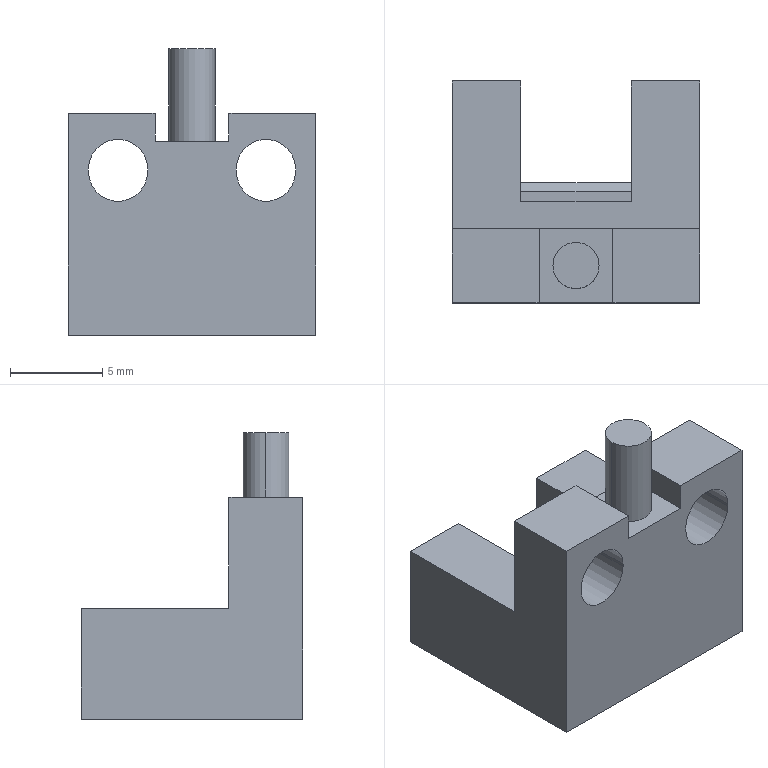Part | SolidWorks | features ICE 1, MBimport 1, MoveFace 1 | 1 solid | 43 faces | box 13.4 x 12 x 15.5 mm | volume 1013 mm3 | plane 37 | cylinder 6 | commonest cylinder face diameters 3.2 x4 2.5 x2
STEP:
#1=CARTESIAN_POINT('',(1.75,-8.,12.5));
#2=VERTEX_POINT('',#1);
#3=CARTESIAN_POINT('',(1.75,-8.,7.5));
#4=VERTEX_POINT('',#3);
#5=CARTESIAN_POINT('',(1.75,-8.,57.5));
#6=DIRECTION('',(0.,0.,-1.));
#7=VECTOR('',#6,1000.);
#8=LINE('',#5,#7);
#9=EDGE_CURVE('',#2,#4,#8,.T.);
#10=ORIENTED_EDGE('',*,*,#9,.F.);
#11=CARTESIAN_POINT('',(4.25,-8.,12.5));
#12=VERTEX_POINT('',#11);
#13=CARTESIAN_POINT('',(3.,-8.,12.5));
#14=DIRECTION('',(0.,0.,1.));
#15=DIRECTION('',(1.,0.,0.));
#16=AXIS2_PLACEMENT_3D('',#13,#14,#15);
#17=CIRCLE('',#16,1.25);
#18=EDGE_CURVE('',#12,#2,#17,.T.);
#19=ORIENTED_EDGE('',*,*,#18,.F.);
#20=CARTESIAN_POINT('',(4.25,-8.,7.5));
#21=VERTEX_POINT('',#20);
#22=CARTESIAN_POINT('',(4.25,-8.,57.5));
#23=DIRECTION('',(0.,0.,-1.));
#24=VECTOR('',#23,1000.);
#25=LINE('',#22,#24);
#26=EDGE_CURVE('',#12,#21,#25,.T.);
#27=ORIENTED_EDGE('',*,*,#26,.T.);
#28=CARTESIAN_POINT('',(3.,-8.,7.5));
#29=DIRECTION('',(0.,0.,1.));
#30=DIRECTION('',(-1.,0.,0.));
#31=AXIS2_PLACEMENT_3D('',#28,#29,#30);
#32=CIRCLE('',#31,1.25);
#33=EDGE_CURVE('',#21,#4,#32,.T.);
#34=ORIENTED_EDGE('',*,*,#33,.T.);
#35=EDGE_LOOP('',(#10,#19,#27,#34));
#36=FACE_OUTER_BOUND('',#35,.T.);
#37=CARTESIAN_POINT('',(3.,-8.,57.5));
#38=DIRECTION('',(0.,0.,-1.));
#39=DIRECTION('',(-1.,0.,0.));
#40=AXIS2_PLACEMENT_3D('',#37,#38,#39);
#41=CYLINDRICAL_SURFACE('',#40,1.25);
#42=ADVANCED_FACE('',(#36),#41,.T.);
#43=ORIENTED_EDGE('',*,*,#26,.F.);
#44=CARTESIAN_POINT('',(3.,-8.,12.5));
#45=DIRECTION('',(0.,0.,1.));
#46=DIRECTION('',(1.,0.,0.));
#47=AXIS2_PLACEMENT_3D('',#44,#45,#46);
#48=CIRCLE('',#47,1.25);
#49=EDGE_CURVE('',#2,#12,#48,.T.);
#50=ORIENTED_EDGE('',*,*,#49,.F.);
#51=ORIENTED_EDGE('',*,*,#9,.T.);
#52=CARTESIAN_POINT('',(3.,-8.,7.5));
#53=DIRECTION('',(0.,0.,1.));
#54=DIRECTION('',(-1.,0.,0.));
#55=AXIS2_PLACEMENT_3D('',#52,#53,#54);
#56=CIRCLE('',#55,1.25);
#57=EDGE_CURVE('',#4,#21,#56,.T.);
#58=ORIENTED_EDGE('',*,*,#57,.T.);
#59=EDGE_LOOP('',(#43,#50,#51,#58));
#60=FACE_OUTER_BOUND('',#59,.T.);
#61=CARTESIAN_POINT('',(3.,-8.,57.5));
#62=DIRECTION('',(0.,0.,-1.));
#63=DIRECTION('',(-1.,0.,0.));
#64=AXIS2_PLACEMENT_3D('',#61,#62,#63);
#65=CYLINDRICAL_SURFACE('',#64,1.25);
#66=ADVANCED_FACE('',(#60),#65,.T.);
#67=CARTESIAN_POINT('',(5.,-6.,7.5));
#68=VERTEX_POINT('',#67);
#69=CARTESIAN_POINT('',(1.,-6.,7.5));
#70=VERTEX_POINT('',#69);
#71=CARTESIAN_POINT('',(1.,-6.,7.5));
#72=DIRECTION('',(-1.,0.,0.));
#73=VECTOR('',#72,1000.);
#74=LINE('',#71,#73);
#75=EDGE_CURVE('',#68,#70,#74,.T.);
#76=ORIENTED_EDGE('',*,*,#75,.T.);
#77=CARTESIAN_POINT('',(1.,-10.,7.5));
#78=VERTEX_POINT('',#77);
#79=CARTESIAN_POINT('',(1.,-10.,7.5));
#80=DIRECTION('',(0.,1.,0.));
#81=VECTOR('',#80,1000.);
#82=LINE('',#79,#81);
#83=EDGE_CURVE('',#78,#70,#82,.T.);
#84=ORIENTED_EDGE('',*,*,#83,.F.);
#85=CARTESIAN_POINT('',(5.,-10.,7.5));
#86=VERTEX_POINT('',#85);
#87=CARTESIAN_POINT('',(1.,-10.,7.5));
#88=DIRECTION('',(-1.,0.,0.));
#89=VECTOR('',#88,1000.);
#90=LINE('',#87,#89);
#91=EDGE_CURVE('',#86,#78,#90,.T.);
#92=ORIENTED_EDGE('',*,*,#91,.F.);
#93=CARTESIAN_POINT('',(5.,-10.,7.5));
#94=DIRECTION('',(0.,1.,0.));
#95=VECTOR('',#94,1000.);
#96=LINE('',#93,#95);
#97=EDGE_CURVE('',#86,#68,#96,.T.);
#98=ORIENTED_EDGE('',*,*,#97,.T.);
#99=EDGE_LOOP('',(#76,#84,#92,#98));
#100=FACE_OUTER_BOUND('',#99,.T.);
#101=ORIENTED_EDGE('',*,*,#57,.F.);
#102=ORIENTED_EDGE('',*,*,#33,.F.);
#103=EDGE_LOOP('',(#101,#102));
#104=FACE_BOUND('',#103,.T.);
#105=CARTESIAN_POINT('',(1.,-10.,7.5));
#106=DIRECTION('',(0.,0.,-1.));
#107=DIRECTION('',(0.,-1.,0.));
#108=AXIS2_PLACEMENT_3D('',#105,#106,#107);
#109=PLANE('',#108);
#110=ADVANCED_FACE('',(#100,#104),#109,.F.);
#111=CARTESIAN_POINT('',(5.,-10.,9.));
#112=VERTEX_POINT('',#111);
#113=CARTESIAN_POINT('',(5.,-6.,9.));
#114=VERTEX_POINT('',#113);
#115=CARTESIAN_POINT('',(5.,-10.,9.));
#116=DIRECTION('',(0.,1.,0.));
#117=VECTOR('',#116,1000.);
#118=LINE('',#115,#117);
#119=EDGE_CURVE('',#112,#114,#118,.T.);
#120=ORIENTED_EDGE('',*,*,#119,.F.);
#121=CARTESIAN_POINT('',(9.7,-10.,9.));
#122=VERTEX_POINT('',#121);
#123=CARTESIAN_POINT('',(9.7,-10.,9.));
#124=DIRECTION('',(1.,0.,0.));
#125=VECTOR('',#124,1000.);
#126=LINE('',#123,#125);
#127=EDGE_CURVE('',#112,#122,#126,.T.);
#128=ORIENTED_EDGE('',*,*,#127,.T.);
#129=CARTESIAN_POINT('',(9.7,-6.,9.));
#130=VERTEX_POINT('',#129);
#131=CARTESIAN_POINT('',(9.7,-10.,9.));
#132=DIRECTION('',(0.,1.,0.));
#133=VECTOR('',#132,1000.);
#134=LINE('',#131,#133);
#135=EDGE_CURVE('',#122,#130,#134,.T.);
#136=ORIENTED_EDGE('',*,*,#135,.T.);
#137=CARTESIAN_POINT('',(9.7,-6.,9.));
#138=DIRECTION('',(-1.,0.,0.));
#139=VECTOR('',#138,1000.);
#140=LINE('',#137,#139);
#141=EDGE_CURVE('',#130,#114,#140,.T.);
#142=ORIENTED_EDGE('',*,*,#141,.T.);
#143=EDGE_LOOP('',(#120,#128,#136,#142));
#144=FACE_OUTER_BOUND('',#143,.T.);
#145=CARTESIAN_POINT('',(9.7,-6.,9.));
#146=DIRECTION('',(0.,0.,1.));
#147=DIRECTION('',(1.,0.,0.));
#148=AXIS2_PLACEMENT_3D('',#145,#146,#147);
#149=PLANE('',#148);
#150=ADVANCED_FACE('',(#144),#149,.T.);
#151=CARTESIAN_POINT('',(0.,-4.5,-3.));
#152=VERTEX_POINT('',#151);
#153=CARTESIAN_POINT('',(0.,2.,-3.));
#154=VERTEX_POINT('',#153);
#155=CARTESIAN_POINT('',(0.,-3.5,-3.));
#156=DIRECTION('',(0.,1.,0.));
#157=VECTOR('',#156,1000.);
#158=LINE('',#155,#157);
#159=EDGE_CURVE('',#152,#154,#158,.T.);
#160=ORIENTED_EDGE('',*,*,#159,.T.);
#161=CARTESIAN_POINT('',(0.,2.,3.));
#162=VERTEX_POINT('',#161);
#163=CARTESIAN_POINT('',(0.,2.,3.));
#164=DIRECTION('',(0.,0.,-1.));
#165=VECTOR('',#164,1000.);
#166=LINE('',#163,#165);
#167=EDGE_CURVE('',#162,#154,#166,.T.);
#168=ORIENTED_EDGE('',*,*,#167,.F.);
#169=CARTESIAN_POINT('',(0.,-4.5,3.));
#170=VERTEX_POINT('',#169);
#171=CARTESIAN_POINT('',(0.,-3.5,3.));
#172=DIRECTION('',(0.,1.,0.));
#173=VECTOR('',#172,1000.);
#174=LINE('',#171,#173);
#175=EDGE_CURVE('',#170,#162,#174,.T.);
#176=ORIENTED_EDGE('',*,*,#175,.F.);
#177=CARTESIAN_POINT('',(0.,-4.5,2.5));
#178=VERTEX_POINT('',#177);
#179=CARTESIAN_POINT('',(0.,-4.5,3.));
#180=DIRECTION('',(0.,0.,1.));
#181=VECTOR('',#180,1000.);
#182=LINE('',#179,#181);
#183=EDGE_CURVE('',#178,#170,#182,.T.);
#184=ORIENTED_EDGE('',*,*,#183,.F.);
#185=CARTESIAN_POINT('',(0.,-4.,2.5));
#186=VERTEX_POINT('',#185);
#187=CARTESIAN_POINT('',(0.,-4.5,2.5));
#188=DIRECTION('',(0.,1.,0.));
#189=VECTOR('',#188,1000.);
#190=LINE('',#187,#189);
#191=EDGE_CURVE('',#178,#186,#190,.T.);
#192=ORIENTED_EDGE('',*,*,#191,.T.);
#193=CARTESIAN_POINT('',(0.,-3.5,2.));
#194=VERTEX_POINT('',#193);
#195=CARTESIAN_POINT('',(0.,-4.,2.5));
#196=DIRECTION('',(0.,0.7071,-0.7071));
#197=VECTOR('',#196,1000.);
#198=LINE('',#195,#197);
#199=EDGE_CURVE('',#186,#194,#198,.T.);
#200=ORIENTED_EDGE('',*,*,#199,.T.);
#201=CARTESIAN_POINT('',(0.,-3.5,-2.));
#202=VERTEX_POINT('',#201);
#203=CARTESIAN_POINT('',(0.,-3.5,3.));
#204=DIRECTION('',(0.,0.,-1.));
#205=VECTOR('',#204,1000.);
#206=LINE('',#203,#205);
#207=EDGE_CURVE('',#194,#202,#206,.T.);
#208=ORIENTED_EDGE('',*,*,#207,.T.);
#209=CARTESIAN_POINT('',(0.,-4.,-2.5));
#210=VERTEX_POINT('',#209);
#211=CARTESIAN_POINT('',(0.,-1.,0.5));
#212=DIRECTION('',(0.,-0.7071,-0.7071));
#213=VECTOR('',#212,1000.);
#214=LINE('',#211,#213);
#215=EDGE_CURVE('',#202,#210,#214,.T.);
#216=ORIENTED_EDGE('',*,*,#215,.T.);
#217=CARTESIAN_POINT('',(0.,-4.5,-2.5));
#218=VERTEX_POINT('',#217);
#219=CARTESIAN_POINT('',(0.,-4.5,-2.5));
#220=DIRECTION('',(0.,1.,0.));
#221=VECTOR('',#220,1000.);
#222=LINE('',#219,#221);
#223=EDGE_CURVE('',#218,#210,#222,.T.);
#224=ORIENTED_EDGE('',*,*,#223,.F.);
#225=CARTESIAN_POINT('',(0.,-4.5,-3.));
#226=DIRECTION('',(0.,0.,1.));
#227=VECTOR('',#226,1000.);
#228=LINE('',#225,#227);
#229=EDGE_CURVE('',#152,#218,#228,.T.);
#230=ORIENTED_EDGE('',*,*,#229,.F.);
#231=EDGE_LOOP('',(#160,#168,#176,#184,#192,#200,#208,#216,#224,#230));
#232=FACE_OUTER_BOUND('',#231,.T.);
#233=CARTESIAN_POINT('',(0.,-0.6,0.4));
#234=VERTEX_POINT('',#233);
#235=CARTESIAN_POINT('',(0.,-0.6,-0.4));
#236=VERTEX_POINT('',#235);
#237=CARTESIAN_POINT('',(0.,-0.6,0.4));
#238=DIRECTION('',(0.,0.,-1.));
#239=VECTOR('',#238,1000.);
#240=LINE('',#237,#239);
#241=EDGE_CURVE('',#234,#236,#240,.T.);
#242=ORIENTED_EDGE('',*,*,#241,.F.);
#243=CARTESIAN_POINT('',(0.,0.6,0.4));
#244=VERTEX_POINT('',#243);
#245=CARTESIAN_POINT('',(0.,-0.6,0.4));
#246=DIRECTION('',(0.,-1.,0.));
#247=VECTOR('',#246,1000.);
#248=LINE('',#245,#247);
#249=EDGE_CURVE('',#244,#234,#248,.T.);
#250=ORIENTED_EDGE('',*,*,#249,.F.);
#251=CARTESIAN_POINT('',(0.,0.6,-0.4));
#252=VERTEX_POINT('',#251);
#253=CARTESIAN_POINT('',(0.,0.6,0.4));
#254=DIRECTION('',(0.,0.,1.));
#255=VECTOR('',#254,1000.);
#256=LINE('',#253,#255);
#257=EDGE_CURVE('',#252,#244,#256,.T.);
#258=ORIENTED_EDGE('',*,*,#257,.F.);
#259=CARTESIAN_POINT('',(0.,-0.6,-0.4));
#260=DIRECTION('',(0.,1.,0.));
#261=VECTOR('',#260,1000.);
#262=LINE('',#259,#261);
#263=EDGE_CURVE('',#236,#252,#262,.T.);
#264=ORIENTED_EDGE('',*,*,#263,.F.);
#265=EDGE_LOOP('',(#242,#250,#258,#264));
#266=FACE_BOUND('',#265,.T.);
#267=CARTESIAN_POINT('',(0.,-3.5,3.));
#268=DIRECTION('',(-1.,0.,0.));
#269=DIRECTION('',(0.,0.,1.));
#270=AXIS2_PLACEMENT_3D('',#267,#268,#269);
#271=PLANE('',#270);
#272=ADVANCED_FACE('',(#232,#266),#271,.F.);
#273=CARTESIAN_POINT('',(-3.7,2.,-3.));
#274=VERTEX_POINT('',#273);
#275=CARTESIAN_POINT('',(0.,2.,-3.));
#276=DIRECTION('',(-1.,0.,0.));
#277=VECTOR('',#276,1000.);
#278=LINE('',#275,#277);
#279=EDGE_CURVE('',#154,#274,#278,.T.);
#280=ORIENTED_EDGE('',*,*,#279,.T.);
#281=CARTESIAN_POINT('',(-3.7,2.,3.));
#282=VERTEX_POINT('',#281);
#283=CARTESIAN_POINT('',(-3.7,2.,3.));
#284=DIRECTION('',(0.,0.,-1.));
#285=VECTOR('',#284,1000.);
#286=LINE('',#283,#285);
#287=EDGE_CURVE('',#282,#274,#286,.T.);
#288=ORIENTED_EDGE('',*,*,#287,.F.);
#289=CARTESIAN_POINT('',(0.,2.,3.));
#290=DIRECTION('',(-1.,0.,0.));
#291=VECTOR('',#290,1000.);
#292=LINE('',#289,#291);
#293=EDGE_CURVE('',#162,#282,#292,.T.);
#294=ORIENTED_EDGE('',*,*,#293,.F.);
#295=ORIENTED_EDGE('',*,*,#167,.T.);
#296=EDGE_LOOP('',(#280,#288,#294,#295));
#297=FACE_OUTER_BOUND('',#296,.T.);
#298=CARTESIAN_POINT('',(0.,2.,3.));
#299=DIRECTION('',(0.,-1.,0.));
#300=DIRECTION('',(0.,0.,-1.));
#301=AXIS2_PLACEMENT_3D('',#298,#299,#300);
#302=PLANE('',#301);
#303=ADVANCED_FACE('',(#297),#302,.F.);
#304=CARTESIAN_POINT('',(-3.7,-10.,-3.));
#305=VERTEX_POINT('',#304);
#306=CARTESIAN_POINT('',(-3.7,2.,-3.));
#307=DIRECTION('',(0.,-1.,0.));
#308=VECTOR('',#307,1000.);
#309=LINE('',#306,#308);
#310=EDGE_CURVE('',#274,#305,#309,.T.);
#311=ORIENTED_EDGE('',*,*,#310,.T.);
#312=CARTESIAN_POINT('',(-3.7,-10.,9.));
#313=VERTEX_POINT('',#312);
#314=CARTESIAN_POINT('',(-3.7,-10.,3.));
#315=DIRECTION('',(0.,0.,-1.));
#316=VECTOR('',#315,1000.);
#317=LINE('',#314,#316);
#318=EDGE_CURVE('',#313,#305,#317,.T.);
#319=ORIENTED_EDGE('',*,*,#318,.F.);
#320=CARTESIAN_POINT('',(-3.7,-6.,9.));
#321=VERTEX_POINT('',#320);
#322=CARTESIAN_POINT('',(-3.7,-10.,9.));
#323=DIRECTION('',(0.,-1.,0.));
#324=VECTOR('',#323,1000.);
#325=LINE('',#322,#324);
#326=EDGE_CURVE('',#321,#313,#325,.T.);
#327=ORIENTED_EDGE('',*,*,#326,.F.);
#328=CARTESIAN_POINT('',(-3.7,-6.,3.));
#329=VERTEX_POINT('',#328);
#330=CARTESIAN_POINT('',(-3.7,-6.,9.));
#331=DIRECTION('',(0.,0.,-1.));
#332=VECTOR('',#331,1000.);
#333=LINE('',#330,#332);
#334=EDGE_CURVE('',#321,#329,#333,.T.);
#335=ORIENTED_EDGE('',*,*,#334,.T.);
#336=CARTESIAN_POINT('',(-3.7,2.,3.));
#337=DIRECTION('',(0.,-1.,0.));
#338=VECTOR('',#337,1000.);
#339=LINE('',#336,#338);
#340=EDGE_CURVE('',#282,#329,#339,.T.);
#341=ORIENTED_EDGE('',*,*,#340,.F.);
#342=ORIENTED_EDGE('',*,*,#287,.T.);
#343=EDGE_LOOP('',(#311,#319,#327,#335,#341,#342));
#344=FACE_OUTER_BOUND('',#343,.T.);
#345=CARTESIAN_POINT('',(-3.7,2.,3.));
#346=DIRECTION('',(1.,0.,0.));
#347=DIRECTION('',(0.,1.,0.));
#348=AXIS2_PLACEMENT_3D('',#345,#346,#347);
#349=PLANE('',#348);
#350=ADVANCED_FACE('',(#344),#349,.F.);
#351=ORIENTED_EDGE('',*,*,#127,.F.);
#352=CARTESIAN_POINT('',(5.,-10.,9.));
#353=DIRECTION('',(0.,0.,-1.));
#354=VECTOR('',#353,1000.);
#355=LINE('',#352,#354);
#356=EDGE_CURVE('',#112,#86,#355,.T.);
#357=ORIENTED_EDGE('',*,*,#356,.T.);
#358=ORIENTED_EDGE('',*,*,#91,.T.);
#359=CARTESIAN_POINT('',(1.,-10.,9.));
#360=VERTEX_POINT('',#359);
#361=CARTESIAN_POINT('',(1.,-10.,9.));
#362=DIRECTION('',(0.,0.,1.));
#363=VECTOR('',#362,1000.);
#364=LINE('',#361,#363);
#365=EDGE_CURVE('',#78,#360,#364,.T.);
#366=ORIENTED_EDGE('',*,*,#365,.T.);
#367=CARTESIAN_POINT('',(9.7,-10.,9.));
#368=DIRECTION('',(1.,0.,0.));
#369=VECTOR('',#368,1000.);
#370=LINE('',#367,#369);
#371=EDGE_CURVE('',#313,#360,#370,.T.);
#372=ORIENTED_EDGE('',*,*,#371,.F.);
#373=ORIENTED_EDGE('',*,*,#318,.T.);
#374=CARTESIAN_POINT('',(9.7,-10.,-3.));
#375=VERTEX_POINT('',#374);
#376=CARTESIAN_POINT('',(-3.7,-10.,-3.));
#377=DIRECTION('',(1.,0.,0.));
#378=VECTOR('',#377,1000.);
#379=LINE('',#376,#378);
#380=EDGE_CURVE('',#305,#375,#379,.T.);
#381=ORIENTED_EDGE('',*,*,#380,.T.);
#382=CARTESIAN_POINT('',(9.7,-10.,3.));
#383=DIRECTION('',(0.,0.,-1.));
#384=VECTOR('',#383,1000.);
#385=LINE('',#382,#384);
#386=EDGE_CURVE('',#122,#375,#385,.T.);
#387=ORIENTED_EDGE('',*,*,#386,.F.);
#388=EDGE_LOOP('',(#351,#357,#358,#366,#372,#373,#381,#387));
#389=FACE_OUTER_BOUND('',#388,.T.);
#390=CARTESIAN_POINT('',(-2.6,-10.,5.85));
#391=VERTEX_POINT('',#390);
#392=CARTESIAN_POINT('',(-2.6,-10.,6.));
#393=VERTEX_POINT('',#392);
#394=CARTESIAN_POINT('',(-2.6,-10.,5.85));
#395=DIRECTION('',(0.,0.,1.));
#396=VECTOR('',#395,1000.);
#397=LINE('',#394,#396);
#398=EDGE_CURVE('',#391,#393,#397,.T.);
#399=ORIENTED_EDGE('',*,*,#398,.T.);
#400=CARTESIAN_POINT('',(0.6,-10.,6.));
#401=VERTEX_POINT('',#400);
#402=CARTESIAN_POINT('',(-1.,-10.,6.));
#403=DIRECTION('',(0.,1.,0.));
#404=DIRECTION('',(1.,0.,0.));
#405=AXIS2_PLACEMENT_3D('',#402,#403,#404);
#406=CIRCLE('',#405,1.6);
#407=EDGE_CURVE('',#393,#401,#406,.T.);
#408=ORIENTED_EDGE('',*,*,#407,.T.);
#409=CARTESIAN_POINT('',(0.6,-10.,5.85));
#410=VERTEX_POINT('',#409);
#411=CARTESIAN_POINT('',(0.6,-10.,5.85));
#412=DIRECTION('',(0.,0.,-1.));
#413=VECTOR('',#412,1000.);
#414=LINE('',#411,#413);
#415=EDGE_CURVE('',#401,#410,#414,.T.);
#416=ORIENTED_EDGE('',*,*,#415,.T.);
#417=CARTESIAN_POINT('',(-1.,-10.,5.85));
#418=DIRECTION('',(0.,1.,0.));
#419=DIRECTION('',(1.,0.,0.));
#420=AXIS2_PLACEMENT_3D('',#417,#418,#419);
#421=CIRCLE('',#420,1.6);
#422=EDGE_CURVE('',#410,#391,#421,.T.);
#423=ORIENTED_EDGE('',*,*,#422,.T.);
#424=EDGE_LOOP('',(#399,#408,#416,#423));
#425=FACE_BOUND('',#424,.T.);
#426=CARTESIAN_POINT('',(8.6,-10.,6.));
#427=VERTEX_POINT('',#426);
#428=CARTESIAN_POINT('',(8.6,-10.,5.85));
#429=VERTEX_POINT('',#428);
#430=CARTESIAN_POINT('',(8.6,-10.,5.85));
#431=DIRECTION('',(0.,0.,-1.));
#432=VECTOR('',#431,1000.);
#433=LINE('',#430,#432);
#434=EDGE_CURVE('',#427,#429,#433,.T.);
#435=ORIENTED_EDGE('',*,*,#434,.T.);
#436=CARTESIAN_POINT('',(5.4,-10.,5.85));
#437=VERTEX_POINT('',#436);
#438=CARTESIAN_POINT('',(7.,-10.,5.85));
#439=DIRECTION('',(0.,1.,0.));
#440=DIRECTION('',(-1.,0.,0.));
#441=AXIS2_PLACEMENT_3D('',#438,#439,#440);
#442=CIRCLE('',#441,1.6);
#443=EDGE_CURVE('',#429,#437,#442,.T.);
#444=ORIENTED_EDGE('',*,*,#443,.T.);
#445=CARTESIAN_POINT('',(5.4,-10.,6.));
#446=VERTEX_POINT('',#445);
#447=CARTESIAN_POINT('',(5.4,-10.,5.85));
#448=DIRECTION('',(0.,0.,1.));
#449=VECTOR('',#448,1000.);
#450=LINE('',#447,#449);
#451=EDGE_CURVE('',#437,#446,#450,.T.);
#452=ORIENTED_EDGE('',*,*,#451,.T.);
#453=CARTESIAN_POINT('',(7.,-10.,6.));
#454=DIRECTION('',(0.,1.,0.));
#455=DIRECTION('',(-1.,0.,0.));
#456=AXIS2_PLACEMENT_3D('',#453,#454,#455);
#457=CIRCLE('',#456,1.6);
#458=EDGE_CURVE('',#446,#427,#457,.T.);
#459=ORIENTED_EDGE('',*,*,#458,.T.);
#460=EDGE_LOOP('',(#435,#444,#452,#459));
#461=FACE_BOUND('',#460,.T.);
#462=CARTESIAN_POINT('',(-3.7,-10.,3.));
#463=DIRECTION('',(0.,1.,0.));
#464=DIRECTION('',(1.,0.,0.));
#465=AXIS2_PLACEMENT_3D('',#462,#463,#464);
#466=PLANE('',#465);
#467=ADVANCED_FACE('',(#389,#425,#461),#466,.F.);
#468=CARTESIAN_POINT('',(9.7,2.,-3.));
#469=VERTEX_POINT('',#468);
#470=CARTESIAN_POINT('',(9.7,-10.,-3.));
#471=DIRECTION('',(0.,1.,0.));
#472=VECTOR('',#471,1000.);
#473=LINE('',#470,#472);
#474=EDGE_CURVE('',#375,#469,#473,.T.);
#475=ORIENTED_EDGE('',*,*,#474,.T.);
#476=CARTESIAN_POINT('',(9.7,2.,3.));
#477=VERTEX_POINT('',#476);
#478=CARTESIAN_POINT('',(9.7,2.,3.));
#479=DIRECTION('',(0.,0.,-1.));
#480=VECTOR('',#479,1000.);
#481=LINE('',#478,#480);
#482=EDGE_CURVE('',#477,#469,#481,.T.);
#483=ORIENTED_EDGE('',*,*,#482,.F.);
#484=CARTESIAN_POINT('',(9.7,-6.,3.));
#485=VERTEX_POINT('',#484);
#486=CARTESIAN_POINT('',(9.7,-10.,3.));
#487=DIRECTION('',(0.,1.,0.));
#488=VECTOR('',#487,1000.);
#489=LINE('',#486,#488);
#490=EDGE_CURVE('',#485,#477,#489,.T.);
#491=ORIENTED_EDGE('',*,*,#490,.F.);
#492=CARTESIAN_POINT('',(9.7,-6.,9.));
#493=DIRECTION('',(0.,0.,-1.));
#494=VECTOR('',#493,1000.);
#495=LINE('',#492,#494);
#496=EDGE_CURVE('',#130,#485,#495,.T.);
#497=ORIENTED_EDGE('',*,*,#496,.F.);
#498=ORIENTED_EDGE('',*,*,#135,.F.);
#499=ORIENTED_EDGE('',*,*,#386,.T.);
#500=EDGE_LOOP('',(#475,#483,#491,#497,#498,#499));
#501=FACE_OUTER_BOUND('',#500,.T.);
#502=CARTESIAN_POINT('',(9.7,-10.,3.));
#503=DIRECTION('',(-1.,0.,0.));
#504=DIRECTION('',(0.,0.,1.));
#505=AXIS2_PLACEMENT_3D('',#502,#503,#504);
#506=PLANE('',#505);
#507=ADVANCED_FACE('',(#501),#506,.F.);
#508=CARTESIAN_POINT('',(6.,2.,-3.));
#509=VERTEX_POINT('',#508);
#510=CARTESIAN_POINT('',(9.7,2.,-3.));
#511=DIRECTION('',(-1.,0.,0.));
#512=VECTOR('',#511,1000.);
#513=LINE('',#510,#512);
#514=EDGE_CURVE('',#469,#509,#513,.T.);
#515=ORIENTED_EDGE('',*,*,#514,.T.);
#516=CARTESIAN_POINT('',(6.,2.,3.));
#517=VERTEX_POINT('',#516);
#518=CARTESIAN_POINT('',(6.,2.,3.));
#519=DIRECTION('',(0.,0.,-1.));
#520=VECTOR('',#519,1000.);
#521=LINE('',#518,#520);
#522=EDGE_CURVE('',#517,#509,#521,.T.);
#523=ORIENTED_EDGE('',*,*,#522,.F.);
#524=CARTESIAN_POINT('',(9.7,2.,3.));
#525=DIRECTION('',(-1.,0.,0.));
#526=VECTOR('',#525,1000.);
#527=LINE('',#524,#526);
#528=EDGE_CURVE('',#477,#517,#527,.T.);
#529=ORIENTED_EDGE('',*,*,#528,.F.);
#530=ORIENTED_EDGE('',*,*,#482,.T.);
#531=EDGE_LOOP('',(#515,#523,#529,#530));
#532=FACE_OUTER_BOUND('',#531,.T.);
#533=CARTESIAN_POINT('',(9.7,2.,3.));
#534=DIRECTION('',(0.,-1.,0.));
#535=DIRECTION('',(0.,0.,-1.));
#536=AXIS2_PLACEMENT_3D('',#533,#534,#535);
#537=PLANE('',#536);
#538=ADVANCED_FACE('',(#532),#537,.F.);
#539=CARTESIAN_POINT('',(6.,-4.5,-3.));
#540=VERTEX_POINT('',#539);
#541=CARTESIAN_POINT('',(6.,2.,-3.));
#542=DIRECTION('',(0.,-1.,0.));
#543=VECTOR('',#542,1000.);
#544=LINE('',#541,#543);
#545=EDGE_CURVE('',#509,#540,#544,.T.);
#546=ORIENTED_EDGE('',*,*,#545,.T.);
#547=CARTESIAN_POINT('',(6.,-4.5,-2.5));
#548=VERTEX_POINT('',#547);
#549=CARTESIAN_POINT('',(6.,-4.5,-3.));
#550=DIRECTION('',(0.,0.,-1.));
#551=VECTOR('',#550,1000.);
#552=LINE('',#549,#551);
#553=EDGE_CURVE('',#548,#540,#552,.T.);
#554=ORIENTED_EDGE('',*,*,#553,.F.);
#555=CARTESIAN_POINT('',(6.,-4.,-2.5));
#556=VERTEX_POINT('',#555);
#557=CARTESIAN_POINT('',(6.,-4.5,-2.5));
#558=DIRECTION('',(0.,1.,0.));
#559=VECTOR('',#558,1000.);
#560=LINE('',#557,#559);
#561=EDGE_CURVE('',#548,#556,#560,.T.);
#562=ORIENTED_EDGE('',*,*,#561,.T.);
#563=CARTESIAN_POINT('',(6.,-3.5,-2.));
#564=VERTEX_POINT('',#563);
#565=CARTESIAN_POINT('',(6.,1.75,3.25));
#566=DIRECTION('',(0.,0.7071,0.7071));
#567=VECTOR('',#566,1000.);
#568=LINE('',#565,#567);
#569=EDGE_CURVE('',#556,#564,#568,.T.);
#570=ORIENTED_EDGE('',*,*,#569,.T.);
#571=CARTESIAN_POINT('',(6.,-3.5,2.));
#572=VERTEX_POINT('',#571);
#573=CARTESIAN_POINT('',(6.,-3.5,3.));
#574=DIRECTION('',(0.,0.,-1.));
#575=VECTOR('',#574,1000.);
#576=LINE('',#573,#575);
#577=EDGE_CURVE('',#572,#564,#576,.T.);
#578=ORIENTED_EDGE('',*,*,#577,.F.);
#579=CARTESIAN_POINT('',(6.,-4.,2.5));
#580=VERTEX_POINT('',#579);
#581=CARTESIAN_POINT('',(6.,-1.25,-0.25));
#582=DIRECTION('',(0.,-0.7071,0.7071));
#583=VECTOR('',#582,1000.);
#584=LINE('',#581,#583);
#585=EDGE_CURVE('',#572,#580,#584,.T.);
#586=ORIENTED_EDGE('',*,*,#585,.T.);
#587=CARTESIAN_POINT('',(6.,-4.5,2.5));
#588=VERTEX_POINT('',#587);
#589=CARTESIAN_POINT('',(6.,-4.5,2.5));
#590=DIRECTION('',(0.,1.,0.));
#591=VECTOR('',#590,1000.);
#592=LINE('',#589,#591);
#593=EDGE_CURVE('',#588,#580,#592,.T.);
#594=ORIENTED_EDGE('',*,*,#593,.F.);
#595=CARTESIAN_POINT('',(6.,-4.5,3.));
#596=VERTEX_POINT('',#595);
#597=CARTESIAN_POINT('',(6.,-4.5,3.));
#598=DIRECTION('',(0.,0.,-1.));
#599=VECTOR('',#598,1000.);
#600=LINE('',#597,#599);
#601=EDGE_CURVE('',#596,#588,#600,.T.);
#602=ORIENTED_EDGE('',*,*,#601,.F.);
#603=CARTESIAN_POINT('',(6.,2.,3.));
#604=DIRECTION('',(0.,-1.,0.));
#605=VECTOR('',#604,1000.);
#606=LINE('',#603,#605);
#607=EDGE_CURVE('',#517,#596,#606,.T.);
#608=ORIENTED_EDGE('',*,*,#607,.F.);
#609=ORIENTED_EDGE('',*,*,#522,.T.);
#610=EDGE_LOOP('',(#546,#554,#562,#570,#578,#586,#594,#602,#608,#609));
#611=FACE_OUTER_BOUND('',#610,.T.);
#612=CARTESIAN_POINT('',(6.,-0.6,-0.4));
#613=VERTEX_POINT('',#612);
#614=CARTESIAN_POINT('',(6.,-0.6,0.4));
#615=VERTEX_POINT('',#614);
#616=CARTESIAN_POINT('',(6.,-0.6,-0.4));
#617=DIRECTION('',(0.,0.,1.));
#618=VECTOR('',#617,1000.);
#619=LINE('',#616,#618);
#620=EDGE_CURVE('',#613,#615,#619,.T.);
#621=ORIENTED_EDGE('',*,*,#620,.F.);
#622=CARTESIAN_POINT('',(6.,0.6,-0.4));
#623=VERTEX_POINT('',#622);
#624=CARTESIAN_POINT('',(6.,-0.6,-0.4));
#625=DIRECTION('',(0.,-1.,0.));
#626=VECTOR('',#625,1000.);
#627=LINE('',#624,#626);
#628=EDGE_CURVE('',#623,#613,#627,.T.);
#629=ORIENTED_EDGE('',*,*,#628,.F.);
#630=CARTESIAN_POINT('',(6.,0.6,0.4));
#631=VERTEX_POINT('',#630);
#632=CARTESIAN_POINT('',(6.,0.6,-0.4));
#633=DIRECTION('',(0.,0.,-1.));
#634=VECTOR('',#633,1000.);
#635=LINE('',#632,#634);
#636=EDGE_CURVE('',#631,#623,#635,.T.);
#637=ORIENTED_EDGE('',*,*,#636,.F.);
#638=CARTESIAN_POINT('',(6.,-0.6,0.4));
#639=DIRECTION('',(0.,1.,0.));
#640=VECTOR('',#639,1000.);
#641=LINE('',#638,#640);
#642=EDGE_CURVE('',#615,#631,#641,.T.);
#643=ORIENTED_EDGE('',*,*,#642,.F.);
#644=EDGE_LOOP('',(#621,#629,#637,#643));
#645=FACE_BOUND('',#644,.T.);
#646=CARTESIAN_POINT('',(6.,2.,3.));
#647=DIRECTION('',(1.,0.,0.));
#648=DIRECTION('',(0.,1.,0.));
#649=AXIS2_PLACEMENT_3D('',#646,#647,#648);
#650=PLANE('',#649);
#651=ADVANCED_FACE('',(#611,#645),#650,.F.);
#652=ORIENTED_EDGE('',*,*,#577,.T.);
#653=CARTESIAN_POINT('',(6.,-3.5,-2.));
#654=DIRECTION('',(-1.,0.,0.));
#655=VECTOR('',#654,1000.);
#656=LINE('',#653,#655);
#657=EDGE_CURVE('',#564,#202,#656,.T.);
#658=ORIENTED_EDGE('',*,*,#657,.T.);
#659=ORIENTED_EDGE('',*,*,#207,.F.);
#660=CARTESIAN_POINT('',(6.,-3.5,2.));
#661=DIRECTION('',(1.,0.,0.));
#662=VECTOR('',#661,1000.);
#663=LINE('',#660,#662);
#664=EDGE_CURVE('',#194,#572,#663,.T.);
#665=ORIENTED_EDGE('',*,*,#664,.T.);
#666=EDGE_LOOP('',(#652,#658,#659,#665));
#667=FACE_OUTER_BOUND('',#666,.T.);
#668=CARTESIAN_POINT('',(6.,-3.5,3.));
#669=DIRECTION('',(0.,-1.,0.));
#670=DIRECTION('',(0.,0.,-1.));
#671=AXIS2_PLACEMENT_3D('',#668,#669,#670);
#672=PLANE('',#671);
#673=ADVANCED_FACE('',(#667),#672,.F.);
#674=ORIENTED_EDGE('',*,*,#607,.T.);
#675=CARTESIAN_POINT('',(6.,-4.5,3.));
#676=DIRECTION('',(1.,0.,0.));
#677=VECTOR('',#676,1000.);
#678=LINE('',#675,#677);
#679=EDGE_CURVE('',#170,#596,#678,.T.);
#680=ORIENTED_EDGE('',*,*,#679,.F.);
#681=ORIENTED_EDGE('',*,*,#175,.T.);
#682=ORIENTED_EDGE('',*,*,#293,.T.);
#683=ORIENTED_EDGE('',*,*,#340,.T.);
#684=CARTESIAN_POINT('',(9.7,-6.,3.));
#685=DIRECTION('',(-1.,0.,0.));
#686=VECTOR('',#685,1000.);
#687=LINE('',#684,#686);
#688=EDGE_CURVE('',#485,#329,#687,.T.);
#689=ORIENTED_EDGE('',*,*,#688,.F.);
#690=ORIENTED_EDGE('',*,*,#490,.T.);
#691=ORIENTED_EDGE('',*,*,#528,.T.);
#692=EDGE_LOOP('',(#674,#680,#681,#682,#683,#689,#690,#691));
#693=FACE_OUTER_BOUND('',#692,.T.);
#694=CARTESIAN_POINT('',(0.,2.,3.));
#695=DIRECTION('',(0.,0.,1.));
#696=DIRECTION('',(1.,0.,0.));
#697=AXIS2_PLACEMENT_3D('',#694,#695,#696);
#698=PLANE('',#697);
#699=ADVANCED_FACE('',(#693),#698,.T.);
#700=CARTESIAN_POINT('',(6.,-4.5,-3.));
#701=DIRECTION('',(-1.,0.,0.));
#702=VECTOR('',#701,1000.);
#703=LINE('',#700,#702);
#704=EDGE_CURVE('',#540,#152,#703,.T.);
#705=ORIENTED_EDGE('',*,*,#704,.F.);
#706=ORIENTED_EDGE('',*,*,#545,.F.);
#707=ORIENTED_EDGE('',*,*,#514,.F.);
#708=ORIENTED_EDGE('',*,*,#474,.F.);
#709=ORIENTED_EDGE('',*,*,#380,.F.);
#710=ORIENTED_EDGE('',*,*,#310,.F.);
#711=ORIENTED_EDGE('',*,*,#279,.F.);
#712=ORIENTED_EDGE('',*,*,#159,.F.);
#713=EDGE_LOOP('',(#705,#706,#707,#708,#709,#710,#711,#712));
#714=FACE_OUTER_BOUND('',#713,.T.);
#715=CARTESIAN_POINT('',(0.,2.,-3.));
#716=DIRECTION('',(0.,0.,1.));
#717=DIRECTION('',(1.,0.,0.));
#718=AXIS2_PLACEMENT_3D('',#715,#716,#717);
#719=PLANE('',#718);
#720=ADVANCED_FACE('',(#714),#719,.F.);
#721=ORIENTED_EDGE('',*,*,#75,.F.);
#722=CARTESIAN_POINT('',(5.,-6.,9.));
#723=DIRECTION('',(0.,0.,-1.));
#724=VECTOR('',#723,1000.);
#725=LINE('',#722,#724);
#726=EDGE_CURVE('',#114,#68,#725,.T.);
#727=ORIENTED_EDGE('',*,*,#726,.F.);
#728=ORIENTED_EDGE('',*,*,#141,.F.);
#729=ORIENTED_EDGE('',*,*,#496,.T.);
#730=ORIENTED_EDGE('',*,*,#688,.T.);
#731=ORIENTED_EDGE('',*,*,#334,.F.);
#732=CARTESIAN_POINT('',(1.,-6.,9.));
#733=VERTEX_POINT('',#732);
#734=CARTESIAN_POINT('',(9.7,-6.,9.));
#735=DIRECTION('',(-1.,0.,0.));
#736=VECTOR('',#735,1000.);
#737=LINE('',#734,#736);
#738=EDGE_CURVE('',#733,#321,#737,.T.);
#739=ORIENTED_EDGE('',*,*,#738,.F.);
#740=CARTESIAN_POINT('',(1.,-6.,9.));
#741=DIRECTION('',(0.,0.,1.));
#742=VECTOR('',#741,1000.);
#743=LINE('',#740,#742);
#744=EDGE_CURVE('',#70,#733,#743,.T.);
#745=ORIENTED_EDGE('',*,*,#744,.F.);
#746=EDGE_LOOP('',(#721,#727,#728,#729,#730,#731,#739,#745));
#747=FACE_OUTER_BOUND('',#746,.T.);
#748=CARTESIAN_POINT('',(0.6,-6.,6.));
#749=VERTEX_POINT('',#748);
#750=CARTESIAN_POINT('',(0.6,-6.,5.85));
#751=VERTEX_POINT('',#750);
#752=CARTESIAN_POINT('',(0.6,-6.,5.85));
#753=DIRECTION('',(0.,0.,-1.));
#754=VECTOR('',#753,1000.);
#755=LINE('',#752,#754);
#756=EDGE_CURVE('',#749,#751,#755,.T.);
#757=ORIENTED_EDGE('',*,*,#756,.F.);
#758=CARTESIAN_POINT('',(-2.6,-6.,6.));
#759=VERTEX_POINT('',#758);
#760=CARTESIAN_POINT('',(-1.,-6.,6.));
#761=DIRECTION('',(0.,1.,0.));
#762=DIRECTION('',(1.,0.,0.));
#763=AXIS2_PLACEMENT_3D('',#760,#761,#762);
#764=CIRCLE('',#763,1.6);
#765=EDGE_CURVE('',#759,#749,#764,.T.);
#766=ORIENTED_EDGE('',*,*,#765,.F.);
#767=CARTESIAN_POINT('',(-2.6,-6.,5.85));
#768=VERTEX_POINT('',#767);
#769=CARTESIAN_POINT('',(-2.6,-6.,5.85));
#770=DIRECTION('',(0.,0.,1.));
#771=VECTOR('',#770,1000.);
#772=LINE('',#769,#771);
#773=EDGE_CURVE('',#768,#759,#772,.T.);
#774=ORIENTED_EDGE('',*,*,#773,.F.);
#775=CARTESIAN_POINT('',(-1.,-6.,5.85));
#776=DIRECTION('',(0.,1.,0.));
#777=DIRECTION('',(1.,0.,0.));
#778=AXIS2_PLACEMENT_3D('',#775,#776,#777);
#779=CIRCLE('',#778,1.6);
#780=EDGE_CURVE('',#751,#768,#779,.T.);
#781=ORIENTED_EDGE('',*,*,#780,.F.);
#782=EDGE_LOOP('',(#757,#766,#774,#781));
#783=FACE_BOUND('',#782,.T.);
#784=CARTESIAN_POINT('',(5.4,-6.,5.85));
#785=VERTEX_POINT('',#784);
#786=CARTESIAN_POINT('',(5.4,-6.,6.));
#787=VERTEX_POINT('',#786);
#788=CARTESIAN_POINT('',(5.4,-6.,5.85));
#789=DIRECTION('',(0.,0.,1.));
#790=VECTOR('',#789,1000.);
#791=LINE('',#788,#790);
#792=EDGE_CURVE('',#785,#787,#791,.T.);
#793=ORIENTED_EDGE('',*,*,#792,.F.);
#794=CARTESIAN_POINT('',(8.6,-6.,5.85));
#795=VERTEX_POINT('',#794);
#796=CARTESIAN_POINT('',(7.,-6.,5.85));
#797=DIRECTION('',(0.,1.,0.));
#798=DIRECTION('',(-1.,0.,0.));
#799=AXIS2_PLACEMENT_3D('',#796,#797,#798);
#800=CIRCLE('',#799,1.6);
#801=EDGE_CURVE('',#795,#785,#800,.T.);
#802=ORIENTED_EDGE('',*,*,#801,.F.);
#803=CARTESIAN_POINT('',(8.6,-6.,6.));
#804=VERTEX_POINT('',#803);
#805=CARTESIAN_POINT('',(8.6,-6.,5.85));
#806=DIRECTION('',(0.,0.,-1.));
#807=VECTOR('',#806,1000.);
#808=LINE('',#805,#807);
#809=EDGE_CURVE('',#804,#795,#808,.T.);
#810=ORIENTED_EDGE('',*,*,#809,.F.);
#811=CARTESIAN_POINT('',(7.,-6.,6.));
#812=DIRECTION('',(0.,1.,0.));
#813=DIRECTION('',(-1.,0.,0.));
#814=AXIS2_PLACEMENT_3D('',#811,#812,#813);
#815=CIRCLE('',#814,1.6);
#816=EDGE_CURVE('',#787,#804,#815,.T.);
#817=ORIENTED_EDGE('',*,*,#816,.F.);
#818=EDGE_LOOP('',(#793,#802,#810,#817));
#819=FACE_BOUND('',#818,.T.);
#820=CARTESIAN_POINT('',(9.7,-6.,9.));
#821=DIRECTION('',(0.,-1.,0.));
#822=DIRECTION('',(0.,0.,-1.));
#823=AXIS2_PLACEMENT_3D('',#820,#821,#822);
#824=PLANE('',#823);
#825=ADVANCED_FACE('',(#747,#783,#819),#824,.F.);
#826=CARTESIAN_POINT('',(1.,-10.,9.));
#827=DIRECTION('',(0.,1.,0.));
#828=VECTOR('',#827,1000.);
#829=LINE('',#826,#828);
#830=EDGE_CURVE('',#360,#733,#829,.T.);
#831=ORIENTED_EDGE('',*,*,#830,.T.);
#832=ORIENTED_EDGE('',*,*,#738,.T.);
#833=ORIENTED_EDGE('',*,*,#326,.T.);
#834=ORIENTED_EDGE('',*,*,#371,.T.);
#835=EDGE_LOOP('',(#831,#832,#833,#834));
#836=FACE_OUTER_BOUND('',#835,.T.);
#837=CARTESIAN_POINT('',(9.7,-6.,9.));
#838=DIRECTION('',(0.,0.,1.));
#839=DIRECTION('',(1.,0.,0.));
#840=AXIS2_PLACEMENT_3D('',#837,#838,#839);
#841=PLANE('',#840);
#842=ADVANCED_FACE('',(#836),#841,.T.);
#843=ORIENTED_EDGE('',*,*,#249,.T.);
#844=CARTESIAN_POINT('',(-0.1,-0.6,0.4));
#845=VERTEX_POINT('',#844);
#846=CARTESIAN_POINT('',(-0.1,-0.6,0.4));
#847=DIRECTION('',(1.,0.,0.));
#848=VECTOR('',#847,1000.);
#849=LINE('',#846,#848);
#850=EDGE_CURVE('',#845,#234,#849,.T.);
#851=ORIENTED_EDGE('',*,*,#850,.F.);
#852=CARTESIAN_POINT('',(-0.1,0.6,0.4));
#853=VERTEX_POINT('',#852);
#854=CARTESIAN_POINT('',(-0.1,-0.6,0.4));
#855=DIRECTION('',(0.,-1.,0.));
#856=VECTOR('',#855,1000.);
#857=LINE('',#854,#856);
#858=EDGE_CURVE('',#853,#845,#857,.T.);
#859=ORIENTED_EDGE('',*,*,#858,.F.);
#860=CARTESIAN_POINT('',(-0.1,0.6,0.4));
#861=DIRECTION('',(1.,0.,0.));
#862=VECTOR('',#861,1000.);
#863=LINE('',#860,#862);
#864=EDGE_CURVE('',#853,#244,#863,.T.);
#865=ORIENTED_EDGE('',*,*,#864,.T.);
#866=EDGE_LOOP('',(#843,#851,#859,#865));
#867=FACE_OUTER_BOUND('',#866,.T.);
#868=CARTESIAN_POINT('',(-0.1,-0.6,0.4));
#869=DIRECTION('',(0.,0.,1.));
#870=DIRECTION('',(1.,0.,0.));
#871=AXIS2_PLACEMENT_3D('',#868,#869,#870);
#872=PLANE('',#871);
#873=ADVANCED_FACE('',(#867),#872,.F.);
#874=ORIENTED_EDGE('',*,*,#257,.T.);
#875=ORIENTED_EDGE('',*,*,#864,.F.);
#876=CARTESIAN_POINT('',(-0.1,0.6,-0.4));
#877=VERTEX_POINT('',#876);
#878=CARTESIAN_POINT('',(-0.1,0.6,0.4));
#879=DIRECTION('',(0.,0.,1.));
#880=VECTOR('',#879,1000.);
#881=LINE('',#878,#880);
#882=EDGE_CURVE('',#877,#853,#881,.T.);
#883=ORIENTED_EDGE('',*,*,#882,.F.);
#884=CARTESIAN_POINT('',(-0.1,0.6,-0.4));
#885=DIRECTION('',(1.,0.,0.));
#886=VECTOR('',#885,1000.);
#887=LINE('',#884,#886);
#888=EDGE_CURVE('',#877,#252,#887,.T.);
#889=ORIENTED_EDGE('',*,*,#888,.T.);
#890=EDGE_LOOP('',(#874,#875,#883,#889));
#891=FACE_OUTER_BOUND('',#890,.T.);
#892=CARTESIAN_POINT('',(-0.1,0.6,0.4));
#893=DIRECTION('',(0.,1.,0.));
#894=DIRECTION('',(1.,0.,0.));
#895=AXIS2_PLACEMENT_3D('',#892,#893,#894);
#896=PLANE('',#895);
#897=ADVANCED_FACE('',(#891),#896,.F.);
#898=ORIENTED_EDGE('',*,*,#263,.T.);
#899=ORIENTED_EDGE('',*,*,#888,.F.);
#900=CARTESIAN_POINT('',(-0.1,-0.6,-0.4));
#901=VERTEX_POINT('',#900);
#902=CARTESIAN_POINT('',(-0.1,-0.6,-0.4));
#903=DIRECTION('',(0.,1.,0.));
#904=VECTOR('',#903,1000.);
#905=LINE('',#902,#904);
#906=EDGE_CURVE('',#901,#877,#905,.T.);
#907=ORIENTED_EDGE('',*,*,#906,.F.);
#908=CARTESIAN_POINT('',(-0.1,-0.6,-0.4));
#909=DIRECTION('',(1.,0.,0.));
#910=VECTOR('',#909,1000.);
#911=LINE('',#908,#910);
#912=EDGE_CURVE('',#901,#236,#911,.T.);
#913=ORIENTED_EDGE('',*,*,#912,.T.);
#914=EDGE_LOOP('',(#898,#899,#907,#913));
#915=FACE_OUTER_BOUND('',#914,.T.);
#916=CARTESIAN_POINT('',(-0.1,-0.6,-0.4));
#917=DIRECTION('',(0.,0.,-1.));
#918=DIRECTION('',(0.,-1.,0.));
#919=AXIS2_PLACEMENT_3D('',#916,#917,#918);
#920=PLANE('',#919);
#921=ADVANCED_FACE('',(#915),#920,.F.);
#922=ORIENTED_EDGE('',*,*,#241,.T.);
#923=ORIENTED_EDGE('',*,*,#912,.F.);
#924=CARTESIAN_POINT('',(-0.1,-0.6,0.4));
#925=DIRECTION('',(0.,0.,-1.));
#926=VECTOR('',#925,1000.);
#927=LINE('',#924,#926);
#928=EDGE_CURVE('',#845,#901,#927,.T.);
#929=ORIENTED_EDGE('',*,*,#928,.F.);
#930=ORIENTED_EDGE('',*,*,#850,.T.);
#931=EDGE_LOOP('',(#922,#923,#929,#930));
#932=FACE_OUTER_BOUND('',#931,.T.);
#933=CARTESIAN_POINT('',(-0.1,-0.6,0.4));
#934=DIRECTION('',(0.,-1.,0.));
#935=DIRECTION('',(-1.,0.,0.));
#936=AXIS2_PLACEMENT_3D('',#933,#934,#935);
#937=PLANE('',#936);
#938=ADVANCED_FACE('',(#932),#937,.F.);
#939=ORIENTED_EDGE('',*,*,#858,.T.);
#940=ORIENTED_EDGE('',*,*,#928,.T.);
#941=ORIENTED_EDGE('',*,*,#906,.T.);
#942=ORIENTED_EDGE('',*,*,#882,.T.);
#943=EDGE_LOOP('',(#939,#940,#941,#942));
#944=FACE_OUTER_BOUND('',#943,.T.);
#945=CARTESIAN_POINT('',(-0.1,0.6,0.4));
#946=DIRECTION('',(-1.,0.,0.));
#947=DIRECTION('',(0.,0.,1.));
#948=AXIS2_PLACEMENT_3D('',#945,#946,#947);
#949=PLANE('',#948);
#950=ADVANCED_FACE('',(#944),#949,.F.);
#951=ORIENTED_EDGE('',*,*,#628,.T.);
#952=CARTESIAN_POINT('',(6.1,-0.6,-0.4));
#953=VERTEX_POINT('',#952);
#954=CARTESIAN_POINT('',(6.1,-0.6,-0.4));
#955=DIRECTION('',(-1.,0.,0.));
#956=VECTOR('',#955,1000.);
#957=LINE('',#954,#956);
#958=EDGE_CURVE('',#953,#613,#957,.T.);
#959=ORIENTED_EDGE('',*,*,#958,.F.);
#960=CARTESIAN_POINT('',(6.1,0.6,-0.4));
#961=VERTEX_POINT('',#960);
#962=CARTESIAN_POINT('',(6.1,-0.6,-0.4));
#963=DIRECTION('',(0.,-1.,0.));
#964=VECTOR('',#963,1000.);
#965=LINE('',#962,#964);
#966=EDGE_CURVE('',#961,#953,#965,.T.);
#967=ORIENTED_EDGE('',*,*,#966,.F.);
#968=CARTESIAN_POINT('',(6.1,0.6,-0.4));
#969=DIRECTION('',(-1.,0.,0.));
#970=VECTOR('',#969,1000.);
#971=LINE('',#968,#970);
#972=EDGE_CURVE('',#961,#623,#971,.T.);
#973=ORIENTED_EDGE('',*,*,#972,.T.);
#974=EDGE_LOOP('',(#951,#959,#967,#973));
#975=FACE_OUTER_BOUND('',#974,.T.);
#976=CARTESIAN_POINT('',(6.1,-0.6,-0.4));
#977=DIRECTION('',(0.,0.,-1.));
#978=DIRECTION('',(0.,-1.,0.));
#979=AXIS2_PLACEMENT_3D('',#976,#977,#978);
#980=PLANE('',#979);
#981=ADVANCED_FACE('',(#975),#980,.F.);
#982=ORIENTED_EDGE('',*,*,#636,.T.);
#983=ORIENTED_EDGE('',*,*,#972,.F.);
#984=CARTESIAN_POINT('',(6.1,0.6,0.4));
#985=VERTEX_POINT('',#984);
#986=CARTESIAN_POINT('',(6.1,0.6,-0.4));
#987=DIRECTION('',(0.,0.,-1.));
#988=VECTOR('',#987,1000.);
#989=LINE('',#986,#988);
#990=EDGE_CURVE('',#985,#961,#989,.T.);
#991=ORIENTED_EDGE('',*,*,#990,.F.);
#992=CARTESIAN_POINT('',(6.1,0.6,0.4));
#993=DIRECTION('',(-1.,0.,0.));
#994=VECTOR('',#993,1000.);
#995=LINE('',#992,#994);
#996=EDGE_CURVE('',#985,#631,#995,.T.);
#997=ORIENTED_EDGE('',*,*,#996,.T.);
#998=EDGE_LOOP('',(#982,#983,#991,#997));
#999=FACE_OUTER_BOUND('',#998,.T.);
#1000=CARTESIAN_POINT('',(6.1,0.6,-0.4));
#1001=DIRECTION('',(0.,1.,0.));
#1002=DIRECTION('',(1.,0.,0.));
#1003=AXIS2_PLACEMENT_3D('',#1000,#1001,#1002);
#1004=PLANE('',#1003);
#1005=ADVANCED_FACE('',(#999),#1004,.F.);
#1006=ORIENTED_EDGE('',*,*,#642,.T.);
#1007=ORIENTED_EDGE('',*,*,#996,.F.);
#1008=CARTESIAN_POINT('',(6.1,-0.6,0.4));
#1009=VERTEX_POINT('',#1008);
#1010=CARTESIAN_POINT('',(6.1,-0.6,0.4));
#1011=DIRECTION('',(0.,1.,0.));
#1012=VECTOR('',#1011,1000.);
#1013=LINE('',#1010,#1012);
#1014=EDGE_CURVE('',#1009,#985,#1013,.T.);
#1015=ORIENTED_EDGE('',*,*,#1014,.F.);
#1016=CARTESIAN_POINT('',(6.1,-0.6,0.4));
#1017=DIRECTION('',(-1.,0.,0.));
#1018=VECTOR('',#1017,1000.);
#1019=LINE('',#1016,#1018);
#1020=EDGE_CURVE('',#1009,#615,#1019,.T.);
#1021=ORIENTED_EDGE('',*,*,#1020,.T.);
#1022=EDGE_LOOP('',(#1006,#1007,#1015,#1021));
#1023=FACE_OUTER_BOUND('',#1022,.T.);
#1024=CARTESIAN_POINT('',(6.1,-0.6,0.4));
#1025=DIRECTION('',(0.,0.,1.));
#1026=DIRECTION('',(1.,0.,0.));
#1027=AXIS2_PLACEMENT_3D('',#1024,#1025,#1026);
#1028=PLANE('',#1027);
#1029=ADVANCED_FACE('',(#1023),#1028,.F.);
#1030=ORIENTED_EDGE('',*,*,#620,.T.);
#1031=ORIENTED_EDGE('',*,*,#1020,.F.);
#1032=CARTESIAN_POINT('',(6.1,-0.6,-0.4));
#1033=DIRECTION('',(0.,0.,1.));
#1034=VECTOR('',#1033,1000.);
#1035=LINE('',#1032,#1034);
#1036=EDGE_CURVE('',#953,#1009,#1035,.T.);
#1037=ORIENTED_EDGE('',*,*,#1036,.F.);
#1038=ORIENTED_EDGE('',*,*,#958,.T.);
#1039=EDGE_LOOP('',(#1030,#1031,#1037,#1038));
#1040=FACE_OUTER_BOUND('',#1039,.T.);
#1041=CARTESIAN_POINT('',(6.1,-0.6,-0.4));
#1042=DIRECTION('',(0.,-1.,0.));
#1043=DIRECTION('',(0.,0.,-1.));
#1044=AXIS2_PLACEMENT_3D('',#1041,#1042,#1043);
#1045=PLANE('',#1044);
#1046=ADVANCED_FACE('',(#1040),#1045,.F.);
#1047=ORIENTED_EDGE('',*,*,#966,.T.);
#1048=ORIENTED_EDGE('',*,*,#1036,.T.);
#1049=ORIENTED_EDGE('',*,*,#1014,.T.);
#1050=ORIENTED_EDGE('',*,*,#990,.T.);
#1051=EDGE_LOOP('',(#1047,#1048,#1049,#1050));
#1052=FACE_OUTER_BOUND('',#1051,.T.);
#1053=CARTESIAN_POINT('',(6.1,0.6,-0.4));
#1054=DIRECTION('',(1.,0.,0.));
#1055=DIRECTION('',(0.,1.,0.));
#1056=AXIS2_PLACEMENT_3D('',#1053,#1054,#1055);
#1057=PLANE('',#1056);
#1058=ADVANCED_FACE('',(#1052),#1057,.F.);
#1059=ORIENTED_EDGE('',*,*,#223,.T.);
#1060=CARTESIAN_POINT('',(6.,-4.,-2.5));
#1061=DIRECTION('',(1.,0.,0.));
#1062=VECTOR('',#1061,1000.);
#1063=LINE('',#1060,#1062);
#1064=EDGE_CURVE('',#210,#556,#1063,.T.);
#1065=ORIENTED_EDGE('',*,*,#1064,.T.);
#1066=ORIENTED_EDGE('',*,*,#561,.F.);
#1067=CARTESIAN_POINT('',(6.,-4.5,-2.5));
#1068=DIRECTION('',(1.,0.,0.));
#1069=VECTOR('',#1068,1000.);
#1070=LINE('',#1067,#1069);
#1071=EDGE_CURVE('',#218,#548,#1070,.T.);
#1072=ORIENTED_EDGE('',*,*,#1071,.F.);
#1073=EDGE_LOOP('',(#1059,#1065,#1066,#1072));
#1074=FACE_OUTER_BOUND('',#1073,.T.);
#1075=CARTESIAN_POINT('',(6.,-4.5,-2.5));
#1076=DIRECTION('',(0.,0.,1.));
#1077=DIRECTION('',(1.,0.,0.));
#1078=AXIS2_PLACEMENT_3D('',#1075,#1076,#1077);
#1079=PLANE('',#1078);
#1080=ADVANCED_FACE('',(#1074),#1079,.F.);
#1081=ORIENTED_EDGE('',*,*,#553,.T.);
#1082=ORIENTED_EDGE('',*,*,#704,.T.);
#1083=ORIENTED_EDGE('',*,*,#229,.T.);
#1084=ORIENTED_EDGE('',*,*,#1071,.T.);
#1085=EDGE_LOOP('',(#1081,#1082,#1083,#1084));
#1086=FACE_OUTER_BOUND('',#1085,.T.);
#1087=CARTESIAN_POINT('',(6.,-4.5,-2.5));
#1088=DIRECTION('',(0.,-1.,0.));
#1089=DIRECTION('',(0.,0.,-1.));
#1090=AXIS2_PLACEMENT_3D('',#1087,#1088,#1089);
#1091=PLANE('',#1090);
#1092=ADVANCED_FACE('',(#1086),#1091,.F.);
#1093=ORIENTED_EDGE('',*,*,#593,.T.);
#1094=CARTESIAN_POINT('',(6.,-4.,2.5));
#1095=DIRECTION('',(-1.,0.,0.));
#1096=VECTOR('',#1095,1000.);
#1097=LINE('',#1094,#1096);
#1098=EDGE_CURVE('',#580,#186,#1097,.T.);
#1099=ORIENTED_EDGE('',*,*,#1098,.T.);
#1100=ORIENTED_EDGE('',*,*,#191,.F.);
#1101=CARTESIAN_POINT('',(6.,-4.5,2.5));
#1102=DIRECTION('',(-1.,0.,0.));
#1103=VECTOR('',#1102,1000.);
#1104=LINE('',#1101,#1103);
#1105=EDGE_CURVE('',#588,#178,#1104,.T.);
#1106=ORIENTED_EDGE('',*,*,#1105,.F.);
#1107=EDGE_LOOP('',(#1093,#1099,#1100,#1106));
#1108=FACE_OUTER_BOUND('',#1107,.T.);
#1109=CARTESIAN_POINT('',(6.,-4.5,2.5));
#1110=DIRECTION('',(0.,0.,-1.));
#1111=DIRECTION('',(-1.,0.,0.));
#1112=AXIS2_PLACEMENT_3D('',#1109,#1110,#1111);
#1113=PLANE('',#1112);
#1114=ADVANCED_FACE('',(#1108),#1113,.F.);
#1115=ORIENTED_EDGE('',*,*,#601,.T.);
#1116=ORIENTED_EDGE('',*,*,#1105,.T.);
#1117=ORIENTED_EDGE('',*,*,#183,.T.);
#1118=ORIENTED_EDGE('',*,*,#679,.T.);
#1119=EDGE_LOOP('',(#1115,#1116,#1117,#1118));
#1120=FACE_OUTER_BOUND('',#1119,.T.);
#1121=CARTESIAN_POINT('',(6.,-4.5,2.5));
#1122=DIRECTION('',(0.,1.,0.));
#1123=DIRECTION('',(1.,0.,0.));
#1124=AXIS2_PLACEMENT_3D('',#1121,#1122,#1123);
#1125=PLANE('',#1124);
#1126=ADVANCED_FACE('',(#1120),#1125,.T.);
#1127=ORIENTED_EDGE('',*,*,#726,.T.);
#1128=ORIENTED_EDGE('',*,*,#97,.F.);
#1129=ORIENTED_EDGE('',*,*,#356,.F.);
#1130=ORIENTED_EDGE('',*,*,#119,.T.);
#1131=EDGE_LOOP('',(#1127,#1128,#1129,#1130));
#1132=FACE_OUTER_BOUND('',#1131,.T.);
#1133=CARTESIAN_POINT('',(5.,-10.,9.));
#1134=DIRECTION('',(1.,0.,0.));
#1135=DIRECTION('',(0.,1.,0.));
#1136=AXIS2_PLACEMENT_3D('',#1133,#1134,#1135);
#1137=PLANE('',#1136);
#1138=ADVANCED_FACE('',(#1132),#1137,.F.);
#1139=ORIENTED_EDGE('',*,*,#744,.T.);
#1140=ORIENTED_EDGE('',*,*,#830,.F.);
#1141=ORIENTED_EDGE('',*,*,#365,.F.);
#1142=ORIENTED_EDGE('',*,*,#83,.T.);
#1143=EDGE_LOOP('',(#1139,#1140,#1141,#1142));
#1144=FACE_OUTER_BOUND('',#1143,.T.);
#1145=CARTESIAN_POINT('',(1.,-10.,9.));
#1146=DIRECTION('',(-1.,0.,0.));
#1147=DIRECTION('',(0.,0.,1.));
#1148=AXIS2_PLACEMENT_3D('',#1145,#1146,#1147);
#1149=PLANE('',#1148);
#1150=ADVANCED_FACE('',(#1144),#1149,.F.);
#1151=ORIENTED_EDGE('',*,*,#801,.T.);
#1152=CARTESIAN_POINT('',(5.4,-10.,5.85));
#1153=DIRECTION('',(0.,1.,0.));
#1154=VECTOR('',#1153,1000.);
#1155=LINE('',#1152,#1154);
#1156=EDGE_CURVE('',#437,#785,#1155,.T.);
#1157=ORIENTED_EDGE('',*,*,#1156,.F.);
#1158=ORIENTED_EDGE('',*,*,#443,.F.);
#1159=CARTESIAN_POINT('',(8.6,-10.,5.85));
#1160=DIRECTION('',(0.,1.,0.));
#1161=VECTOR('',#1160,1000.);
#1162=LINE('',#1159,#1161);
#1163=EDGE_CURVE('',#429,#795,#1162,.T.);
#1164=ORIENTED_EDGE('',*,*,#1163,.T.);
#1165=EDGE_LOOP('',(#1151,#1157,#1158,#1164));
#1166=FACE_OUTER_BOUND('',#1165,.T.);
#1167=CARTESIAN_POINT('',(7.,-10.,5.85));
#1168=DIRECTION('',(0.,1.,0.));
#1169=DIRECTION('',(-1.,0.,0.));
#1170=AXIS2_PLACEMENT_3D('',#1167,#1168,#1169);
#1171=CYLINDRICAL_SURFACE('',#1170,1.6);
#1172=ADVANCED_FACE('',(#1166),#1171,.F.);
#1173=ORIENTED_EDGE('',*,*,#809,.T.);
#1174=ORIENTED_EDGE('',*,*,#1163,.F.);
#1175=ORIENTED_EDGE('',*,*,#434,.F.);
#1176=CARTESIAN_POINT('',(8.6,-10.,6.));
#1177=DIRECTION('',(0.,1.,0.));
#1178=VECTOR('',#1177,1000.);
#1179=LINE('',#1176,#1178);
#1180=EDGE_CURVE('',#427,#804,#1179,.T.);
#1181=ORIENTED_EDGE('',*,*,#1180,.T.);
#1182=EDGE_LOOP('',(#1173,#1174,#1175,#1181));
#1183=FACE_OUTER_BOUND('',#1182,.T.);
#1184=CARTESIAN_POINT('',(8.6,-10.,5.85));
#1185=DIRECTION('',(1.,0.,0.));
#1186=DIRECTION('',(0.,0.,1.));
#1187=AXIS2_PLACEMENT_3D('',#1184,#1185,#1186);
#1188=PLANE('',#1187);
#1189=ADVANCED_FACE('',(#1183),#1188,.F.);
#1190=ORIENTED_EDGE('',*,*,#816,.T.);
#1191=ORIENTED_EDGE('',*,*,#1180,.F.);
#1192=ORIENTED_EDGE('',*,*,#458,.F.);
#1193=CARTESIAN_POINT('',(5.4,-10.,6.));
#1194=DIRECTION('',(0.,1.,0.));
#1195=VECTOR('',#1194,1000.);
#1196=LINE('',#1193,#1195);
#1197=EDGE_CURVE('',#446,#787,#1196,.T.);
#1198=ORIENTED_EDGE('',*,*,#1197,.T.);
#1199=EDGE_LOOP('',(#1190,#1191,#1192,#1198));
#1200=FACE_OUTER_BOUND('',#1199,.T.);
#1201=CARTESIAN_POINT('',(7.,-10.,6.));
#1202=DIRECTION('',(0.,1.,0.));
#1203=DIRECTION('',(-1.,0.,0.));
#1204=AXIS2_PLACEMENT_3D('',#1201,#1202,#1203);
#1205=CYLINDRICAL_SURFACE('',#1204,1.6);
#1206=ADVANCED_FACE('',(#1200),#1205,.F.);
#1207=ORIENTED_EDGE('',*,*,#792,.T.);
#1208=ORIENTED_EDGE('',*,*,#1197,.F.);
#1209=ORIENTED_EDGE('',*,*,#451,.F.);
#1210=ORIENTED_EDGE('',*,*,#1156,.T.);
#1211=EDGE_LOOP('',(#1207,#1208,#1209,#1210));
#1212=FACE_OUTER_BOUND('',#1211,.T.);
#1213=CARTESIAN_POINT('',(5.4,-10.,5.85));
#1214=DIRECTION('',(-1.,0.,0.));
#1215=DIRECTION('',(0.,1.,0.));
#1216=AXIS2_PLACEMENT_3D('',#1213,#1214,#1215);
#1217=PLANE('',#1216);
#1218=ADVANCED_FACE('',(#1212),#1217,.F.);
#1219=ORIENTED_EDGE('',*,*,#765,.T.);
#1220=CARTESIAN_POINT('',(0.6,-10.,6.));
#1221=DIRECTION('',(0.,1.,0.));
#1222=VECTOR('',#1221,1000.);
#1223=LINE('',#1220,#1222);
#1224=EDGE_CURVE('',#401,#749,#1223,.T.);
#1225=ORIENTED_EDGE('',*,*,#1224,.F.);
#1226=ORIENTED_EDGE('',*,*,#407,.F.);
#1227=CARTESIAN_POINT('',(-2.6,-10.,6.));
#1228=DIRECTION('',(0.,1.,0.));
#1229=VECTOR('',#1228,1000.);
#1230=LINE('',#1227,#1229);
#1231=EDGE_CURVE('',#393,#759,#1230,.T.);
#1232=ORIENTED_EDGE('',*,*,#1231,.T.);
#1233=EDGE_LOOP('',(#1219,#1225,#1226,#1232));
#1234=FACE_OUTER_BOUND('',#1233,.T.);
#1235=CARTESIAN_POINT('',(-1.,-10.,6.));
#1236=DIRECTION('',(0.,1.,0.));
#1237=DIRECTION('',(-1.,0.,0.));
#1238=AXIS2_PLACEMENT_3D('',#1235,#1236,#1237);
#1239=CYLINDRICAL_SURFACE('',#1238,1.6);
#1240=ADVANCED_FACE('',(#1234),#1239,.F.);
#1241=ORIENTED_EDGE('',*,*,#773,.T.);
#1242=ORIENTED_EDGE('',*,*,#1231,.F.);
#1243=ORIENTED_EDGE('',*,*,#398,.F.);
#1244=CARTESIAN_POINT('',(-2.6,-10.,5.85));
#1245=DIRECTION('',(0.,1.,0.));
#1246=VECTOR('',#1245,1000.);
#1247=LINE('',#1244,#1246);
#1248=EDGE_CURVE('',#391,#768,#1247,.T.);
#1249=ORIENTED_EDGE('',*,*,#1248,.T.);
#1250=EDGE_LOOP('',(#1241,#1242,#1243,#1249));
#1251=FACE_OUTER_BOUND('',#1250,.T.);
#1252=CARTESIAN_POINT('',(-2.6,-10.,5.85));
#1253=DIRECTION('',(-1.,0.,0.));
#1254=DIRECTION('',(0.,1.,0.));
#1255=AXIS2_PLACEMENT_3D('',#1252,#1253,#1254);
#1256=PLANE('',#1255);
#1257=ADVANCED_FACE('',(#1251),#1256,.F.);
#1258=ORIENTED_EDGE('',*,*,#780,.T.);
#1259=ORIENTED_EDGE('',*,*,#1248,.F.);
#1260=ORIENTED_EDGE('',*,*,#422,.F.);
#1261=CARTESIAN_POINT('',(0.6,-10.,5.85));
#1262=DIRECTION('',(0.,1.,0.));
#1263=VECTOR('',#1262,1000.);
#1264=LINE('',#1261,#1263);
#1265=EDGE_CURVE('',#410,#751,#1264,.T.);
#1266=ORIENTED_EDGE('',*,*,#1265,.T.);
#1267=EDGE_LOOP('',(#1258,#1259,#1260,#1266));
#1268=FACE_OUTER_BOUND('',#1267,.T.);
#1269=CARTESIAN_POINT('',(-1.,-10.,5.85));
#1270=DIRECTION('',(0.,1.,0.));
#1271=DIRECTION('',(-1.,0.,0.));
#1272=AXIS2_PLACEMENT_3D('',#1269,#1270,#1271);
#1273=CYLINDRICAL_SURFACE('',#1272,1.6);
#1274=ADVANCED_FACE('',(#1268),#1273,.F.);
#1275=ORIENTED_EDGE('',*,*,#756,.T.);
#1276=ORIENTED_EDGE('',*,*,#1265,.F.);
#1277=ORIENTED_EDGE('',*,*,#415,.F.);
#1278=ORIENTED_EDGE('',*,*,#1224,.T.);
#1279=EDGE_LOOP('',(#1275,#1276,#1277,#1278));
#1280=FACE_OUTER_BOUND('',#1279,.T.);
#1281=CARTESIAN_POINT('',(0.6,-10.,5.85));
#1282=DIRECTION('',(1.,0.,0.));
#1283=DIRECTION('',(0.,1.,0.));
#1284=AXIS2_PLACEMENT_3D('',#1281,#1282,#1283);
#1285=PLANE('',#1284);
#1286=ADVANCED_FACE('',(#1280),#1285,.F.);
#1287=ORIENTED_EDGE('',*,*,#215,.F.);
#1288=ORIENTED_EDGE('',*,*,#657,.F.);
#1289=ORIENTED_EDGE('',*,*,#569,.F.);
#1290=ORIENTED_EDGE('',*,*,#1064,.F.);
#1291=EDGE_LOOP('',(#1287,#1288,#1289,#1290));
#1292=FACE_OUTER_BOUND('',#1291,.T.);
#1293=CARTESIAN_POINT('',(6.,-4.,-2.5));
#1294=DIRECTION('',(0.,-0.7071,0.7071));
#1295=DIRECTION('',(-1.,0.,0.));
#1296=AXIS2_PLACEMENT_3D('',#1293,#1294,#1295);
#1297=PLANE('',#1296);
#1298=ADVANCED_FACE('',(#1292),#1297,.F.);
#1299=ORIENTED_EDGE('',*,*,#585,.F.);
#1300=ORIENTED_EDGE('',*,*,#664,.F.);
#1301=ORIENTED_EDGE('',*,*,#199,.F.);
#1302=ORIENTED_EDGE('',*,*,#1098,.F.);
#1303=EDGE_LOOP('',(#1299,#1300,#1301,#1302));
#1304=FACE_OUTER_BOUND('',#1303,.T.);
#1305=CARTESIAN_POINT('',(6.,-4.,2.5));
#1306=DIRECTION('',(0.,-0.7071,-0.7071));
#1307=DIRECTION('',(0.,-0.7071,0.7071));
#1308=AXIS2_PLACEMENT_3D('',#1305,#1306,#1307);
#1309=PLANE('',#1308);
#1310=ADVANCED_FACE('',(#1304),#1309,.F.);
#1311=ORIENTED_EDGE('',*,*,#18,.T.);
#1312=ORIENTED_EDGE('',*,*,#49,.T.);
#1313=EDGE_LOOP('',(#1311,#1312));
#1314=FACE_OUTER_BOUND('',#1313,.T.);
#1315=CARTESIAN_POINT('',(3.,-8.,12.5));
#1316=DIRECTION('',(0.,0.,1.));
#1317=DIRECTION('',(1.,0.,0.));
#1318=AXIS2_PLACEMENT_3D('',#1315,#1316,#1317);
#1319=PLANE('',#1318);
#1320=ADVANCED_FACE('',(#1314),#1319,.T.);
#1321=CLOSED_SHELL('',(#42,#66,#110,#150,#272,#303,#350,#467,#507,#538,#651,#673,#699,#720,#825,#842,#873,#897,#921,#938,#950,#981,#1005,#1029,#1046,#1058,#1080,#1092,#1114,#1126,#1138,#1150,#1172,#1189,#1206,#1218,#1240,#1257,#1274,#1286,#1298,#1310,#1320));
#1322=MANIFOLD_SOLID_BREP('',#1321);
#1323=CARTESIAN_POINT('',(0.,0.,0.));
#1324=DIRECTION('',(0.,0.,1.));
#1325=DIRECTION('',(1.,0.,0.));
#1326=AXIS2_PLACEMENT_3D('',#1323,#1324,#1325);
#1327=(LENGTH_UNIT()NAMED_UNIT(*)SI_UNIT(.MILLI.,.METRE.));
#1328=UNCERTAINTY_MEASURE_WITH_UNIT(LENGTH_MEASURE(0.00001),#1327,'','');
#1329=(NAMED_UNIT(*)PLANE_ANGLE_UNIT()SI_UNIT($,.RADIAN.));
#1330=(NAMED_UNIT(*)SI_UNIT($,.STERADIAN.)SOLID_ANGLE_UNIT());
#1331=(GEOMETRIC_REPRESENTATION_CONTEXT(3)GLOBAL_UNCERTAINTY_ASSIGNED_CONTEXT((#1328))GLOBAL_UNIT_ASSIGNED_CONTEXT((#1327,#1329,#1330))REPRESENTATION_CONTEXT('',''));
#1332=ADVANCED_BREP_SHAPE_REPRESENTATION('',(#1322,#1326),#1331);